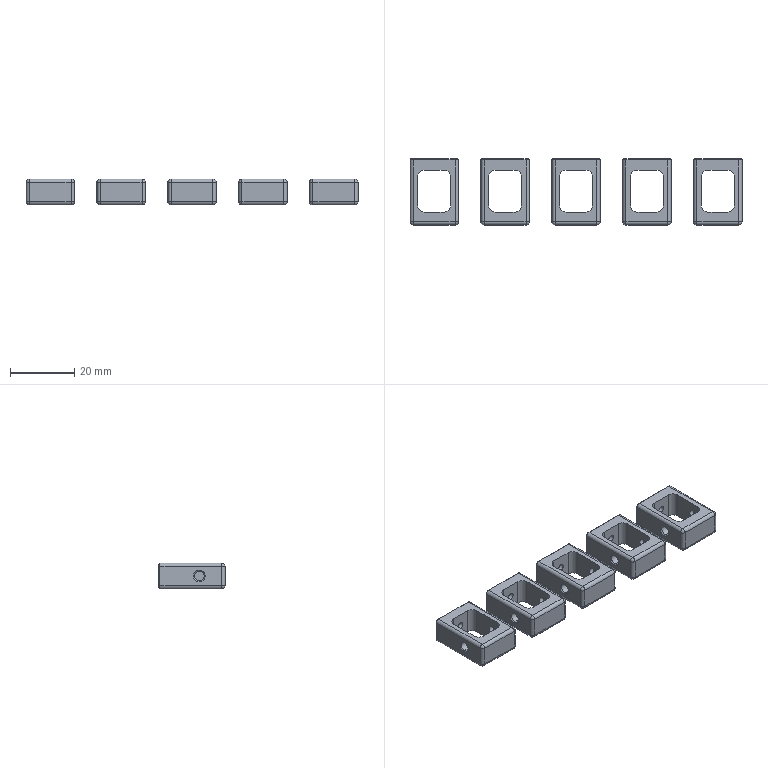NC program | NX | posted with a generic post | part box 103 x 20.5 x 8 mm
Lines 19 to 1022 of 9732:
(ZLEVEL_PROFILE , TOOL : D6)
N36 T12 M6
N38 G54
N40 G17 G0 G90 X20.275 Y-3.15 S9500 M3
N42 G43 Z30. H12
N44 Z1.5
N46 G94 G1 X24. Z1.305 F1000.
N48 Y3.65 Z0.948
N50 X20. Z0.739
N52 Y-3.15 Z0.382
N54 X24. Z0.173
N56 Y3.65 Z-0.184
N58 X20. Z-0.393
N60 Y0.25 Z-0.571
N62 Y-3.15 F3000.
N64 X24.
N66 Y3.65
N68 X20.
N70 Y0.25
N72 Y-3.15 Z-0.661
N74 X24. Z-0.767
N76 Y3.65 Z-0.947
N78 X20. Z-1.053
N80 Y0.25 Z-1.143
N82 Y-3.15 Z-1.233
N84 X24. Z-1.339
N86 Y3.65 Z-1.519
N88 X20. Z-1.624
N90 Y0.25 Z-1.714
N92 Y-3.15 Z-1.804
N94 X24. Z-1.91
N96 Y3.65 Z-2.09
N98 X20. Z-2.196
N100 Y0.25 Z-2.286
N102 Y-3.15 Z-2.376
N104 X24. Z-2.481
N106 Y3.65 Z-2.661
N108 X20. Z-2.767
N110 Y0.25 Z-2.857
N112 Y-3.15 Z-2.947
N114 X24. Z-3.053
N116 Y3.65 Z-3.233
N118 X20. Z-3.339
N120 Y0.25 Z-3.429
N122 Y-3.15 Z-3.519
N124 X24. Z-3.624
N126 Y3.65 Z-3.804
N128 X20. Z-3.91
N130 Y0.25 Z-4.
N132 Y-3.15 Z-4.09
N134 X24. Z-4.196
N136 Y3.65 Z-4.376
N138 X20. Z-4.481
N140 Y0.25 Z-4.571
N142 Y-3.15 Z-4.661
N144 X24. Z-4.767
N146 Y3.65 Z-4.947
N148 X20. Z-5.053
N150 Y0.25 Z-5.143
N152 Y-3.15 Z-5.233
N154 X24. Z-5.339
N156 Y3.65 Z-5.519
N158 X20. Z-5.624
N160 Y0.25 Z-5.714
N162 Y-3.15 Z-5.804
N164 X24. Z-5.91
N166 Y3.65 Z-6.09
N168 X20. Z-6.196
N170 Y0.25 Z-6.286
N172 Y-3.15 Z-6.376
N174 X24. Z-6.481
N176 Y3.65 Z-6.661
N178 X20. Z-6.767
N180 Y0.25 Z-6.857
N182 Y-3.15 Z-6.947
N184 X24. Z-7.053
N186 Y3.65 Z-7.233
N188 X20. Z-7.339
N190 Y0.25 Z-7.429
N192 Y-3.15 Z-7.519
N194 X24. Z-7.624
N196 Y3.65 Z-7.804
N198 X20. Z-7.91
N200 Y0.25 Z-8.
N202 Y-3.15
N204 X24.
N206 Y3.65
N208 X20.
N210 Y0.25
N212 Z-6.5
N214 G0 Z53.
N216 X1.725 Y3.65
N218 Z1.5
N220 G1 X-2. Z1.305 F1000.
N222 Y-3.15 Z0.948
N224 X2. Z0.739
N226 Y3.65 Z0.382
N228 X-2. Z0.173
N230 Y-3.15 Z-0.184
N232 X2. Z-0.393
N234 Y0.25 Z-0.571
N236 Y3.65 F3000.
N238 X-2.
N240 Y-3.15
N242 X2.
N244 Y0.25
N246 Y3.65 Z-0.661
N248 X-2. Z-0.767
N250 Y-3.15 Z-0.947
N252 X2. Z-1.053
N254 Y0.25 Z-1.143
N256 Y3.65 Z-1.233
N258 X-2. Z-1.339
N260 Y-3.15 Z-1.519
N262 X2. Z-1.624
N264 Y0.25 Z-1.714
N266 Y3.65 Z-1.804
N268 X-2. Z-1.91
N270 Y-3.15 Z-2.09
N272 X2. Z-2.196
N274 Y0.25 Z-2.286
N276 Y3.65 Z-2.376
N278 X-2. Z-2.481
N280 Y-3.15 Z-2.661
N282 X2. Z-2.767
N284 Y0.25 Z-2.857
N286 Y3.65 Z-2.947
N288 X-2. Z-3.053
N290 Y-3.15 Z-3.233
N292 X2. Z-3.339
N294 Y0.25 Z-3.429
N296 Y3.65 Z-3.519
N298 X-2. Z-3.624
N300 Y-3.15 Z-3.804
N302 X2. Z-3.91
N304 Y0.25 Z-4.
N306 Y3.65 Z-4.09
N308 X-2. Z-4.196
N310 Y-3.15 Z-4.376
N312 X2. Z-4.481
N314 Y0.25 Z-4.571
N316 Y3.65 Z-4.661
N318 X-2. Z-4.767
N320 Y-3.15 Z-4.947
N322 X2. Z-5.053
N324 Y0.25 Z-5.143
N326 Y3.65 Z-5.233
N328 X-2. Z-5.339
N330 Y-3.15 Z-5.519
N332 X2. Z-5.624
N334 Y0.25 Z-5.714
N336 Y3.65 Z-5.804
N338 X-2. Z-5.91
N340 Y-3.15 Z-6.09
N342 X2. Z-6.196
N344 Y0.25 Z-6.286
N346 Y3.65 Z-6.376
N348 X-2. Z-6.481
N350 Y-3.15 Z-6.661
N352 X2. Z-6.767
N354 Y0.25 Z-6.857
N356 Y3.65 Z-6.947
N358 X-2. Z-7.053
N360 Y-3.15 Z-7.233
N362 X2. Z-7.339
N364 Y0.25 Z-7.429
N366 Y3.65 Z-7.519
N368 X-2. Z-7.624
N370 Y-3.15 Z-7.804
N372 X2. Z-7.91
N374 Y0.25 Z-8.
N376 Y3.65
N378 X-2.
N380 Y-3.15
N382 X2.
N384 Y0.25
N386 Z-6.5
N388 G0 Z53.
N390 X-20.275 Y3.65
N392 Z1.5
N394 G1 X-24. Z1.305 F1000.
N396 Y-3.15 Z0.948
N398 X-20. Z0.739
N400 Y3.65 Z0.382
N402 X-24. Z0.173
N404 Y-3.15 Z-0.184
N406 X-20. Z-0.393
N408 Y0.25 Z-0.571
N410 Y3.65 F3000.
N412 X-24.
N414 Y-3.15
N416 X-20.
N418 Y0.25
N420 Y3.65 Z-0.661
N422 X-24. Z-0.767
N424 Y-3.15 Z-0.947
N426 X-20. Z-1.053
N428 Y0.25 Z-1.143
N430 Y3.65 Z-1.233
N432 X-24. Z-1.339
N434 Y-3.15 Z-1.519
N436 X-20. Z-1.624
N438 Y0.25 Z-1.714
N440 Y3.65 Z-1.804
N442 X-24. Z-1.91
N444 Y-3.15 Z-2.09
N446 X-20. Z-2.196
N448 Y0.25 Z-2.286
N450 Y3.65 Z-2.376
N452 X-24. Z-2.481
N454 Y-3.15 Z-2.661
N456 X-20. Z-2.767
N458 Y0.25 Z-2.857
N460 Y3.65 Z-2.947
N462 X-24. Z-3.053
N464 Y-3.15 Z-3.233
N466 X-20. Z-3.339
N468 Y0.25 Z-3.429
N470 Y3.65 Z-3.519
N472 X-24. Z-3.624
N474 Y-3.15 Z-3.804
N476 X-20. Z-3.91
N478 Y0.25 Z-4.
N480 Y3.65 Z-4.09
N482 X-24. Z-4.196
N484 Y-3.15 Z-4.376
N486 X-20. Z-4.481
N488 Y0.25 Z-4.571
N490 Y3.65 Z-4.661
N492 X-24. Z-4.767
N494 Y-3.15 Z-4.947
N496 X-20. Z-5.053
N498 Y0.25 Z-5.143
N500 Y3.65 Z-5.233
N502 X-24. Z-5.339
N504 Y-3.15 Z-5.519
N506 X-20. Z-5.624
N508 Y0.25 Z-5.714
N510 Y3.65 Z-5.804
N512 X-24. Z-5.91
N514 Y-3.15 Z-6.09
N516 X-20. Z-6.196
N518 Y0.25 Z-6.286
N520 Y3.65 Z-6.376
N522 X-24. Z-6.481
N524 Y-3.15 Z-6.661
N526 X-20. Z-6.767
N528 Y0.25 Z-6.857
N530 Y3.65 Z-6.947
N532 X-24. Z-7.053
N534 Y-3.15 Z-7.233
N536 X-20. Z-7.339
N538 Y0.25 Z-7.429
N540 Y3.65 Z-7.519
N542 X-24. Z-7.624
N544 Y-3.15 Z-7.804
N546 X-20. Z-7.91
N548 Y0.25 Z-8.
N550 Y3.65
N552 X-24.
N554 Y-3.15
N556 X-20.
N558 Y0.25
N560 Z-6.5
N562 G0 Z53.
N564 X-45.725 Y-3.15
N566 Z1.5
N568 G1 X-42. Z1.305 F1000.
N570 Y3.65 Z0.948
N572 X-46. Z0.739
N574 Y-3.15 Z0.382
N576 X-42. Z0.173
N578 Y3.65 Z-0.184
N580 X-46. Z-0.393
N582 Y0.25 Z-0.571
N584 Y-3.15 F3000.
N586 X-42.
N588 Y3.65
N590 X-46.
N592 Y0.25
N594 Y-3.15 Z-0.661
N596 X-42. Z-0.767
N598 Y3.65 Z-0.947
N600 X-46. Z-1.053
N602 Y0.25 Z-1.143
N604 Y-3.15 Z-1.233
N606 X-42. Z-1.339
N608 Y3.65 Z-1.519
N610 X-46. Z-1.624
N612 Y0.25 Z-1.714
N614 Y-3.15 Z-1.804
N616 X-42. Z-1.91
N618 Y3.65 Z-2.09
N620 X-46. Z-2.196
N622 Y0.25 Z-2.286
N624 Y-3.15 Z-2.376
N626 X-42. Z-2.481
N628 Y3.65 Z-2.661
N630 X-46. Z-2.767
N632 Y0.25 Z-2.857
N634 Y-3.15 Z-2.947
N636 X-42. Z-3.053
N638 Y3.65 Z-3.233
N640 X-46. Z-3.339
N642 Y0.25 Z-3.429
N644 Y-3.15 Z-3.519
N646 X-42. Z-3.624
N648 Y3.65 Z-3.804
N650 X-46. Z-3.91
N652 Y0.25 Z-4.
N654 Y-3.15 Z-4.09
N656 X-42. Z-4.196
N658 Y3.65 Z-4.376
N660 X-46. Z-4.481
N662 Y0.25 Z-4.571
N664 Y-3.15 Z-4.661
N666 X-42. Z-4.767
N668 Y3.65 Z-4.947
N670 X-46. Z-5.053
N672 Y0.25 Z-5.143
N674 Y-3.15 Z-5.233
N676 X-42. Z-5.339
N678 Y3.65 Z-5.519
N680 X-46. Z-5.624
N682 Y0.25 Z-5.714
N684 Y-3.15 Z-5.804
N686 X-42. Z-5.91
N688 Y3.65 Z-6.09
N690 X-46. Z-6.196
N692 Y0.25 Z-6.286
N694 Y-3.15 Z-6.376
N696 X-42. Z-6.481
N698 Y3.65 Z-6.661
N700 X-46. Z-6.767
N702 Y0.25 Z-6.857
N704 Y-3.15 Z-6.947
N706 X-42. Z-7.053
N708 Y3.65 Z-7.233
N710 X-46. Z-7.339
N712 Y0.25 Z-7.429
N714 Y-3.15 Z-7.519
N716 X-42. Z-7.624
N718 Y3.65 Z-7.804
N720 X-46. Z-7.91
N722 Y0.25 Z-8.
N724 Y-3.15
N726 X-42.
N728 Y3.65
N730 X-46.
N732 Y0.25
N734 Z-6.5
N736 G0 Z53.
N738 X45.725 Y3.65
N740 Z1.5
N742 G1 X42. Z1.305 F1000.
N744 Y-3.15 Z0.948
N746 X46. Z0.739
N748 Y3.65 Z0.382
N750 X42. Z0.173
N752 Y-3.15 Z-0.184
N754 X46. Z-0.393
N756 Y0.25 Z-0.571
N758 Y3.65 F3000.
N760 X42.
N762 Y-3.15
N764 X46.
N766 Y0.25
N768 Y3.65 Z-0.661
N770 X42. Z-0.767
N772 Y-3.15 Z-0.947
N774 X46. Z-1.053
N776 Y0.25 Z-1.143
N778 Y3.65 Z-1.233
N780 X42. Z-1.339
N782 Y-3.15 Z-1.519
N784 X46. Z-1.624
N786 Y0.25 Z-1.714
N788 Y3.65 Z-1.804
N790 X42. Z-1.91
N792 Y-3.15 Z-2.09
N794 X46. Z-2.196
N796 Y0.25 Z-2.286
N798 Y3.65 Z-2.376
N800 X42. Z-2.481
N802 Y-3.15 Z-2.661
N804 X46. Z-2.767
N806 Y0.25 Z-2.857
N808 Y3.65 Z-2.947
N810 X42. Z-3.053
N812 Y-3.15 Z-3.233
N814 X46. Z-3.339
N816 Y0.25 Z-3.429
N818 Y3.65 Z-3.519
N820 X42. Z-3.624
N822 Y-3.15 Z-3.804
N824 X46. Z-3.91
N826 Y0.25 Z-4.
N828 Y3.65 Z-4.09
N830 X42. Z-4.196
N832 Y-3.15 Z-4.376
N834 X46. Z-4.481
N836 Y0.25 Z-4.571
N838 Y3.65 Z-4.661
N840 X42. Z-4.767
N842 Y-3.15 Z-4.947
N844 X46. Z-5.053
N846 Y0.25 Z-5.143
N848 Y3.65 Z-5.233
N850 X42. Z-5.339
N852 Y-3.15 Z-5.519
N854 X46. Z-5.624
N856 Y0.25 Z-5.714
N858 Y3.65 Z-5.804
N860 X42. Z-5.91
N862 Y-3.15 Z-6.09
N864 X46. Z-6.196
N866 Y0.25 Z-6.286
N868 Y3.65 Z-6.376
N870 X42. Z-6.481
N872 Y-3.15 Z-6.661
N874 X46. Z-6.767
N876 Y0.25 Z-6.857
N878 Y3.65 Z-6.947
N880 X42. Z-7.053
N882 Y-3.15 Z-7.233
N884 X46. Z-7.339
N886 Y0.25 Z-7.429
N888 Y3.65 Z-7.519
N890 X42. Z-7.624
N892 Y-3.15 Z-7.804
N894 X46. Z-7.91
N896 Y0.25 Z-8.
N898 Y3.65
N900 X42.
N902 Y-3.15
N904 X46.
N906 Y0.25
N908 Z-6.5
N910 G0 Z53.
N912 X33.4 Y5.088
N914 Z1.5
N916 G1 Y9.95 Z1.245 F1000.
N918 X33.397 Y10.384 Z1.222
N920 X33.686 Y11.35 Z1.17
N922 X34.265 Y12.175 Z1.117
N924 X34.608 Y12.442 Z1.094
N926 X34.914 Y12.748 Z1.071
N928 X35.602 Y13.142 Z1.03
N930 X36.368 Y13.35 Z0.988
N932 X51.632 Z0.188
N934 X52.398 Y13.142 Z0.147
N936 X53.086 Y12.748 Z0.105
N938 X53.998 Y11.836 Z0.037
N940 X54.392 Y11.148 Z-0.004
N942 X54.6 Y10.382 Z-0.046
N944 Y0.35 Z-0.571
N946 Y-9.25 F3000.
N948 G2 X50.5 Y-13.35 R4.1
N950 G1 X37.5
N952 G2 X33.4 Y-9.25 R4.1
N954 G1 Y9.95
N956 G2 X34.608 Y12.442 R3.129
N958 X36.8 Y13.35 R3.1
N960 G1 X51.2
N962 G2 X53.392 Y12.442 R3.1
N964 G1 X53.692 Y12.142
N966 G2 X54.6 Y9.95 R3.1
N968 G1 Y0.35
N970 Y-9.25 Z-0.633
N972 X54.574 Y-9.709 Z-0.636
N974 X54.497 Y-10.162 Z-0.639
N976 X54.37 Y-10.604 Z-0.642
N978 X54.194 Y-11.029 Z-0.645
N980 X53.972 Y-11.431 Z-0.648
N982 X53.706 Y-11.806 Z-0.651
N984 X53.399 Y-12.149 Z-0.653
N986 X53.056 Y-12.456 Z-0.656
N988 X52.681 Y-12.722 Z-0.659
N990 X52.279 Y-12.944 Z-0.662
N992 X51.854 Y-13.12 Z-0.665
N994 X51.412 Y-13.247 Z-0.668
N996 X50.959 Y-13.324 Z-0.671
N998 X50.5 Y-13.35 Z-0.674
N1000 X37.5 Z-0.757
N1002 X37.041 Y-13.324 Z-0.76
N1004 X36.588 Y-13.247 Z-0.763
N1006 X36.146 Y-13.12 Z-0.766
N1008 X35.721 Y-12.944 Z-0.769
N1010 X35.319 Y-12.722 Z-0.772
N1012 X34.944 Y-12.456 Z-0.775
N1014 X34.601 Y-12.149 Z-0.778
N1016 X34.294 Y-11.806 Z-0.781
N1018 X34.028 Y-11.431 Z-0.784
N1020 X33.806 Y-11.029 Z-0.787
N1022 X33.63 Y-10.604 Z-0.79
N1024 X33.503 Y-10.162 Z-0.793
N1026 X33.426 Y-9.709 Z-0.796
N1028 X33.4 Y-9.25 Z-0.798
N1030 Y9.95 Z-0.921
N1032 X33.421 Y10.307 Z-0.924
N1034 X33.482 Y10.66 Z-0.926
N1036 X33.584 Y11.003 Z-0.928
N1038 X33.725 Y11.331 Z-0.931
N1040 X33.902 Y11.641 Z-0.933
N1042 X34.113 Y11.928 Z-0.935
N1044 X34.356 Y12.19 Z-0.937
N1046 X34.608 Y12.442 Z-0.94
N1048 X34.913 Y12.71 Z-0.942
N1050 X35.25 Y12.935 Z-0.945
N1052 X35.614 Y13.114 Z-0.948
N1054 X35.998 Y13.244 Z-0.95
N1056 X36.395 Y13.323 Z-0.953
N1058 X36.8 Y13.35 Z-0.955
N1060 X51.2 Z-1.048
N1062 X51.605 Y13.323 Z-1.05
N1064 X52.002 Y13.244 Z-1.053
N1066 X52.386 Y13.114 Z-1.055
N1068 X52.75 Y12.935 Z-1.058
N1070 X53.087 Y12.709 Z-1.061
N1072 X53.392 Y12.442 Z-1.063
N1074 X53.692 Y12.142 Z-1.066
N1076 X53.959 Y11.837 Z-1.068
N1078 X54.185 Y11.5 Z-1.071
N1080 X54.364 Y11.136 Z-1.074
N1082 X54.494 Y10.752 Z-1.076
N1084 X54.573 Y10.355 Z-1.079
N1086 X54.6 Y9.95 Z-1.081
N1088 Y0.35 Z-1.143
N1090 Y-9.25 Z-1.204
N1092 X54.574 Y-9.709 Z-1.207
N1094 X54.497 Y-10.162 Z-1.21
N1096 X54.37 Y-10.604 Z-1.213
N1098 X54.194 Y-11.029 Z-1.216
N1100 X53.972 Y-11.431 Z-1.219
N1102 X53.706 Y-11.806 Z-1.222
N1104 X53.399 Y-12.149 Z-1.225
N1106 X53.056 Y-12.456 Z-1.228
N1108 X52.681 Y-12.722 Z-1.231
N1110 X52.279 Y-12.944 Z-1.234
N1112 X51.854 Y-13.12 Z-1.237
N1114 X51.412 Y-13.247 Z-1.24
N1116 X50.959 Y-13.324 Z-1.243
N1118 X50.5 Y-13.35 Z-1.246
N1120 X37.5 Z-1.329
N1122 X37.041 Y-13.324 Z-1.332
N1124 X36.588 Y-13.247 Z-1.335
N1126 X36.146 Y-13.12 Z-1.338
N1128 X35.721 Y-12.944 Z-1.341
N1130 X35.319 Y-12.722 Z-1.343
N1132 X34.944 Y-12.456 Z-1.346
N1134 X34.601 Y-12.149 Z-1.349
N1136 X34.294 Y-11.806 Z-1.352
N1138 X34.028 Y-11.431 Z-1.355
N1140 X33.806 Y-11.029 Z-1.358
N1142 X33.63 Y-10.604 Z-1.361
N1144 X33.503 Y-10.162 Z-1.364
N1146 X33.426 Y-9.709 Z-1.367
N1148 X33.4 Y-9.25 Z-1.37
N1150 Y9.95 Z-1.493
N1152 X33.421 Y10.307 Z-1.495
N1154 X33.482 Y10.66 Z-1.497
N1156 X33.584 Y11.003 Z-1.5
N1158 X33.725 Y11.331 Z-1.502
N1160 X33.902 Y11.641 Z-1.504
N1162 X34.113 Y11.928 Z-1.507
N1164 X34.356 Y12.19 Z-1.509
N1166 X34.608 Y12.442 Z-1.511
N1168 X34.913 Y12.71 Z-1.514
N1170 X35.25 Y12.935 Z-1.516
N1172 X35.614 Y13.114 Z-1.519
N1174 X35.998 Y13.244 Z-1.522
N1176 X36.395 Y13.323 Z-1.524
N1178 X36.8 Y13.35 Z-1.527
N1180 X51.2 Z-1.619
N1182 X51.605 Y13.323 Z-1.622
N1184 X52.002 Y13.244 Z-1.624
N1186 X52.386 Y13.114 Z-1.627
N1188 X52.75 Y12.935 Z-1.629
N1190 X53.087 Y12.709 Z-1.632
N1192 X53.392 Y12.442 Z-1.635
N1194 X53.692 Y12.142 Z-1.637
N1196 X53.959 Y11.837 Z-1.64
N1198 X54.185 Y11.5 Z-1.642
N1200 X54.364 Y11.136 Z-1.645
N1202 X54.494 Y10.752 Z-1.648
N1204 X54.573 Y10.355 Z-1.65
N1206 X54.6 Y9.95 Z-1.653
N1208 Y0.35 Z-1.714
N1210 Y-9.25 Z-1.776
N1212 X54.574 Y-9.709 Z-1.779
N1214 X54.497 Y-10.162 Z-1.782
N1216 X54.37 Y-10.604 Z-1.785
N1218 X54.194 Y-11.029 Z-1.788
N1220 X53.972 Y-11.431 Z-1.79
N1222 X53.706 Y-11.806 Z-1.793
N1224 X53.399 Y-12.149 Z-1.796
N1226 X53.056 Y-12.456 Z-1.799
N1228 X52.681 Y-12.722 Z-1.802
N1230 X52.279 Y-12.944 Z-1.805
N1232 X51.854 Y-13.12 Z-1.808
N1234 X51.412 Y-13.247 Z-1.811
N1236 X50.959 Y-13.324 Z-1.814
N1238 X50.5 Y-13.35 Z-1.817
N1240 X37.5 Z-1.9
N1242 X37.041 Y-13.324 Z-1.903
N1244 X36.588 Y-13.247 Z-1.906
N1246 X36.146 Y-13.12 Z-1.909
N1248 X35.721 Y-12.944 Z-1.912
N1250 X35.319 Y-12.722 Z-1.915
N1252 X34.944 Y-12.456 Z-1.918
N1254 X34.601 Y-12.149 Z-1.921
N1256 X34.294 Y-11.806 Z-1.924
N1258 X34.028 Y-11.431 Z-1.927
N1260 X33.806 Y-11.029 Z-1.93
N1262 X33.63 Y-10.604 Z-1.933
N1264 X33.503 Y-10.162 Z-1.935
N1266 X33.426 Y-9.709 Z-1.938
N1268 X33.4 Y-9.25 Z-1.941
N1270 Y9.95 Z-2.064
N1272 X33.421 Y10.307 Z-2.067
N1274 X33.482 Y10.66 Z-2.069
N1276 X33.584 Y11.003 Z-2.071
N1278 X33.725 Y11.331 Z-2.073
N1280 X33.902 Y11.641 Z-2.076
N1282 X34.113 Y11.928 Z-2.078
N1284 X34.356 Y12.19 Z-2.08
N1286 X34.608 Y12.442 Z-2.083
N1288 X34.913 Y12.71 Z-2.085
N1290 X35.25 Y12.935 Z-2.088
N1292 X35.614 Y13.114 Z-2.09
N1294 X35.998 Y13.244 Z-2.093
N1296 X36.395 Y13.323 Z-2.096
N1298 X36.8 Y13.35 Z-2.098
N1300 X51.2 Z-2.19
N1302 X51.605 Y13.323 Z-2.193
N1304 X52.002 Y13.244 Z-2.196
N1306 X52.386 Y13.114 Z-2.198
N1308 X52.75 Y12.935 Z-2.201
N1310 X53.087 Y12.709 Z-2.203
N1312 X53.392 Y12.442 Z-2.206
N1314 X53.692 Y12.142 Z-2.209
N1316 X53.959 Y11.837 Z-2.211
N1318 X54.185 Y11.5 Z-2.214
N1320 X54.364 Y11.136 Z-2.216
N1322 X54.494 Y10.752 Z-2.219
N1324 X54.573 Y10.355 Z-2.222
N1326 X54.6 Y9.95 Z-2.224
N1328 Y0.35 Z-2.286
N1330 Y-9.25 Z-2.347
N1332 X54.574 Y-9.709 Z-2.35
N1334 X54.497 Y-10.162 Z-2.353
N1336 X54.37 Y-10.604 Z-2.356
N1338 X54.194 Y-11.029 Z-2.359
N1340 X53.972 Y-11.431 Z-2.362
N1342 X53.706 Y-11.806 Z-2.365
N1344 X53.399 Y-12.149 Z-2.368
N1346 X53.056 Y-12.456 Z-2.371
N1348 X52.681 Y-12.722 Z-2.374
N1350 X52.279 Y-12.944 Z-2.377
N1352 X51.854 Y-13.12 Z-2.38
N1354 X51.412 Y-13.247 Z-2.382
N1356 X50.959 Y-13.324 Z-2.385
N1358 X50.5 Y-13.35 Z-2.388
N1360 X37.5 Z-2.472
N1362 X37.041 Y-13.324 Z-2.475
N1364 X36.588 Y-13.247 Z-2.477
N1366 X36.146 Y-13.12 Z-2.48
N1368 X35.721 Y-12.944 Z-2.483
N1370 X35.319 Y-12.722 Z-2.486
N1372 X34.944 Y-12.456 Z-2.489
N1374 X34.601 Y-12.149 Z-2.492
N1376 X34.294 Y-11.806 Z-2.495
N1378 X34.028 Y-11.431 Z-2.498
N1380 X33.806 Y-11.029 Z-2.501
N1382 X33.63 Y-10.604 Z-2.504
N1384 X33.503 Y-10.162 Z-2.507
N1386 X33.426 Y-9.709 Z-2.51
N1388 X33.4 Y-9.25 Z-2.513
N1390 Y9.95 Z-2.636
N1392 X33.421 Y10.307 Z-2.638
N1394 X33.482 Y10.66 Z-2.64
N1396 X33.584 Y11.003 Z-2.643
N1398 X33.725 Y11.331 Z-2.645
N1400 X33.902 Y11.641 Z-2.647
N1402 X34.113 Y11.928 Z-2.649
N1404 X34.356 Y12.19 Z-2.652
N1406 X34.608 Y12.442 Z-2.654
N1408 X34.913 Y12.71 Z-2.657
N1410 X35.25 Y12.935 Z-2.659
N1412 X35.614 Y13.114 Z-2.662
N1414 X35.998 Y13.244 Z-2.664
N1416 X36.395 Y13.323 Z-2.667
N1418 X36.8 Y13.35 Z-2.67
N1420 X51.2 Z-2.762
N1422 X51.605 Y13.323 Z-2.764
N1424 X52.002 Y13.244 Z-2.767
N1426 X52.386 Y13.114 Z-2.77
N1428 X52.75 Y12.935 Z-2.772
N1430 X53.087 Y12.709 Z-2.775
N1432 X53.392 Y12.442 Z-2.777
N1434 X53.692 Y12.142 Z-2.78
N1436 X53.959 Y11.837 Z-2.783
N1438 X54.185 Y11.5 Z-2.785
N1440 X54.364 Y11.136 Z-2.788
N1442 X54.494 Y10.752 Z-2.79
N1444 X54.573 Y10.355 Z-2.793
N1446 X54.6 Y9.95 Z-2.796
N1448 Y0.35 Z-2.857
N1450 Y-9.25 Z-2.919
N1452 X54.574 Y-9.709 Z-2.922
N1454 X54.497 Y-10.162 Z-2.925
N1456 X54.37 Y-10.604 Z-2.927
N1458 X54.194 Y-11.029 Z-2.93
N1460 X53.972 Y-11.431 Z-2.933
N1462 X53.706 Y-11.806 Z-2.936
N1464 X53.399 Y-12.149 Z-2.939
N1466 X53.056 Y-12.456 Z-2.942
N1468 X52.681 Y-12.722 Z-2.945
N1470 X52.279 Y-12.944 Z-2.948
N1472 X51.854 Y-13.12 Z-2.951
N1474 X51.412 Y-13.247 Z-2.954
N1476 X50.959 Y-13.324 Z-2.957
N1478 X50.5 Y-13.35 Z-2.96
N1480 X37.5 Z-3.043
N1482 X37.041 Y-13.324 Z-3.046
N1484 X36.588 Y-13.247 Z-3.049
N1486 X36.146 Y-13.12 Z-3.052
N1488 X35.721 Y-12.944 Z-3.055
N1490 X35.319 Y-12.722 Z-3.058
N1492 X34.944 Y-12.456 Z-3.061
N1494 X34.601 Y-12.149 Z-3.064
N1496 X34.294 Y-11.806 Z-3.067
N1498 X34.028 Y-11.431 Z-3.07
N1500 X33.806 Y-11.029 Z-3.072
N1502 X33.63 Y-10.604 Z-3.075
N1504 X33.503 Y-10.162 Z-3.078
N1506 X33.426 Y-9.709 Z-3.081
N1508 X33.4 Y-9.25 Z-3.084
N1510 Y9.95 Z-3.207
N1512 X33.421 Y10.307 Z-3.209
N1514 X33.482 Y10.66 Z-3.212
N1516 X33.584 Y11.003 Z-3.214
N1518 X33.725 Y11.331 Z-3.216
N1520 X33.902 Y11.641 Z-3.219
N1522 X34.113 Y11.928 Z-3.221
N1524 X34.356 Y12.19 Z-3.223
N1526 X34.608 Y12.442 Z-3.226
N1528 X34.913 Y12.71 Z-3.228
N1530 X35.25 Y12.935 Z-3.231
N1532 X35.614 Y13.114 Z-3.233
N1534 X35.998 Y13.244 Z-3.236
N1536 X36.395 Y13.323 Z-3.238
N1538 X36.8 Y13.35 Z-3.241
N1540 X51.2 Z-3.333
N1542 X51.605 Y13.323 Z-3.336
N1544 X52.002 Y13.244 Z-3.338
N1546 X52.386 Y13.114 Z-3.341
N1548 X52.75 Y12.935 Z-3.344
N1550 X53.087 Y12.709 Z-3.346
N1552 X53.392 Y12.442 Z-3.349
N1554 X53.692 Y12.142 Z-3.352
N1556 X53.959 Y11.837 Z-3.354
N1558 X54.185 Y11.5 Z-3.357
N1560 X54.364 Y11.136 Z-3.359
N1562 X54.494 Y10.752 Z-3.362
N1564 X54.573 Y10.355 Z-3.364
N1566 X54.6 Y9.95 Z-3.367
N1568 Y0.35 Z-3.429
N1570 Y-9.25 Z-3.49
N1572 X54.574 Y-9.709 Z-3.493
N1574 X54.497 Y-10.162 Z-3.496
N1576 X54.37 Y-10.604 Z-3.499
N1578 X54.194 Y-11.029 Z-3.502
N1580 X53.972 Y-11.431 Z-3.505
N1582 X53.706 Y-11.806 Z-3.508
N1584 X53.399 Y-12.149 Z-3.511
N1586 X53.056 Y-12.456 Z-3.514
N1588 X52.681 Y-12.722 Z-3.517
N1590 X52.279 Y-12.944 Z-3.519
N1592 X51.854 Y-13.12 Z-3.522
N1594 X51.412 Y-13.247 Z-3.525
N1596 X50.959 Y-13.324 Z-3.528
N1598 X50.5 Y-13.35 Z-3.531
N1600 X37.5 Z-3.614
N1602 X37.041 Y-13.324 Z-3.617
N1604 X36.588 Y-13.247 Z-3.62
N1606 X36.146 Y-13.12 Z-3.623
N1608 X35.721 Y-12.944 Z-3.626
N1610 X35.319 Y-12.722 Z-3.629
N1612 X34.944 Y-12.456 Z-3.632
N1614 X34.601 Y-12.149 Z-3.635
N1616 X34.294 Y-11.806 Z-3.638
N1618 X34.028 Y-11.431 Z-3.641
N1620 X33.806 Y-11.029 Z-3.644
N1622 X33.63 Y-10.604 Z-3.647
N1624 X33.503 Y-10.162 Z-3.65
N1626 X33.426 Y-9.709 Z-3.653
N1628 X33.4 Y-9.25 Z-3.656
N1630 Y9.95 Z-3.779
N1632 X33.421 Y10.307 Z-3.781
N1634 X33.482 Y10.66 Z-3.783
N1636 X33.584 Y11.003 Z-3.785
N1638 X33.725 Y11.331 Z-3.788
N1640 X33.902 Y11.641 Z-3.79
N1642 X34.113 Y11.928 Z-3.792
N1644 X34.356 Y12.19 Z-3.795
N1646 X34.608 Y12.442 Z-3.797
N1648 X34.913 Y12.71 Z-3.8
N1650 X35.25 Y12.935 Z-3.802
N1652 X35.614 Y13.114 Z-3.805
N1654 X35.998 Y13.244 Z-3.807
N1656 X36.395 Y13.323 Z-3.81
N1658 X36.8 Y13.35 Z-3.812
N1660 X51.2 Z-3.905
N1662 X51.605 Y13.323 Z-3.907
N1664 X52.002 Y13.244 Z-3.91
N1666 X52.386 Y13.114 Z-3.912
N1668 X52.75 Y12.935 Z-3.915
N1670 X53.087 Y12.709 Z-3.918
N1672 X53.392 Y12.442 Z-3.92
N1674 X53.692 Y12.142 Z-3.923
N1676 X53.959 Y11.837 Z-3.926
N1678 X54.185 Y11.5 Z-3.928
N1680 X54.364 Y11.136 Z-3.931
N1682 X54.494 Y10.752 Z-3.933
N1684 X54.573 Y10.355 Z-3.936
N1686 X54.6 Y9.95 Z-3.939
N1688 Y0.35 Z-4.
N1690 Y-9.25 Z-4.061
N1692 X54.574 Y-9.709 Z-4.064
N1694 X54.497 Y-10.162 Z-4.067
N1696 X54.37 Y-10.604 Z-4.07
N1698 X54.194 Y-11.029 Z-4.073
N1700 X53.972 Y-11.431 Z-4.076
N1702 X53.706 Y-11.806 Z-4.079
N1704 X53.399 Y-12.149 Z-4.082
N1706 X53.056 Y-12.456 Z-4.085
N1708 X52.681 Y-12.722 Z-4.088
N1710 X52.279 Y-12.944 Z-4.091
N1712 X51.854 Y-13.12 Z-4.094
N1714 X51.412 Y-13.247 Z-4.097
N1716 X50.959 Y-13.324 Z-4.1
N1718 X50.5 Y-13.35 Z-4.103
N1720 X37.5 Z-4.186
N1722 X37.041 Y-13.324 Z-4.189
N1724 X36.588 Y-13.247 Z-4.192
N1726 X36.146 Y-13.12 Z-4.195
N1728 X35.721 Y-12.944 Z-4.198
N1730 X35.319 Y-12.722 Z-4.201
N1732 X34.944 Y-12.456 Z-4.204
N1734 X34.601 Y-12.149 Z-4.206
N1736 X34.294 Y-11.806 Z-4.209
N1738 X34.028 Y-11.431 Z-4.212
N1740 X33.806 Y-11.029 Z-4.215
N1742 X33.63 Y-10.604 Z-4.218
N1744 X33.503 Y-10.162 Z-4.221
N1746 X33.426 Y-9.709 Z-4.224
N1748 X33.4 Y-9.25 Z-4.227
N1750 Y9.95 Z-4.35
N1752 X33.421 Y10.307 Z-4.352
N1754 X33.482 Y10.66 Z-4.355
N1756 X33.584 Y11.003 Z-4.357
N1758 X33.725 Y11.331 Z-4.359
N1760 X33.902 Y11.641 Z-4.361
N1762 X34.113 Y11.928 Z-4.364
N1764 X34.356 Y12.19 Z-4.366
N1766 X34.608 Y12.442 Z-4.368
N1768 X34.913 Y12.71 Z-4.371
N1770 X35.25 Y12.935 Z-4.374
N1772 X35.614 Y13.114 Z-4.376
N1774 X35.998 Y13.244 Z-4.379
N1776 X36.395 Y13.323 Z-4.381
N1778 X36.8 Y13.35 Z-4.384
N1780 X51.2 Z-4.476
N1782 X51.605 Y13.323 Z-4.479
N1784 X52.002 Y13.244 Z-4.481
N1786 X52.386 Y13.114 Z-4.484
N1788 X52.75 Y12.935 Z-4.486
N1790 X53.087 Y12.709 Z-4.489
N1792 X53.392 Y12.442 Z-4.492
N1794 X53.692 Y12.142 Z-4.494
N1796 X53.959 Y11.837 Z-4.497
N1798 X54.185 Y11.5 Z-4.5
N1800 X54.364 Y11.136 Z-4.502
N1802 X54.494 Y10.752 Z-4.505
N1804 X54.573 Y10.355 Z-4.507
N1806 X54.6 Y9.95 Z-4.51
N1808 Y0.35 Z-4.571
N1810 Y-9.25 Z-4.633
N1812 X54.574 Y-9.709 Z-4.636
N1814 X54.497 Y-10.162 Z-4.639
N1816 X54.37 Y-10.604 Z-4.642
N1818 X54.194 Y-11.029 Z-4.645
N1820 X53.972 Y-11.431 Z-4.648
N1822 X53.706 Y-11.806 Z-4.651
N1824 X53.399 Y-12.149 Z-4.653
N1826 X53.056 Y-12.456 Z-4.656
N1828 X52.681 Y-12.722 Z-4.659
N1830 X52.279 Y-12.944 Z-4.662
N1832 X51.854 Y-13.12 Z-4.665
N1834 X51.412 Y-13.247 Z-4.668
N1836 X50.959 Y-13.324 Z-4.671
N1838 X50.5 Y-13.35 Z-4.674
N1840 X37.5 Z-4.757
N1842 X37.041 Y-13.324 Z-4.76
N1844 X36.588 Y-13.247 Z-4.763
N1846 X36.146 Y-13.12 Z-4.766
N1848 X35.721 Y-12.944 Z-4.769
N1850 X35.319 Y-12.722 Z-4.772
N1852 X34.944 Y-12.456 Z-4.775
N1854 X34.601 Y-12.149 Z-4.778
N1856 X34.294 Y-11.806 Z-4.781
N1858 X34.028 Y-11.431 Z-4.784
N1860 X33.806 Y-11.029 Z-4.787
N1862 X33.63 Y-10.604 Z-4.79
N1864 X33.503 Y-10.162 Z-4.793
N1866 X33.426 Y-9.709 Z-4.796
N1868 X33.4 Y-9.25 Z-4.798
N1870 Y9.95 Z-4.921
N1872 X33.421 Y10.307 Z-4.924
N1874 X33.482 Y10.66 Z-4.926
N1876 X33.584 Y11.003 Z-4.928
N1878 X33.725 Y11.331 Z-4.931
N1880 X33.902 Y11.641 Z-4.933
N1882 X34.113 Y11.928 Z-4.935
N1884 X34.356 Y12.19 Z-4.937
N1886 X34.608 Y12.442 Z-4.94
N1888 X34.913 Y12.71 Z-4.942
N1890 X35.25 Y12.935 Z-4.945
N1892 X35.614 Y13.114 Z-4.948
N1894 X35.998 Y13.244 Z-4.95
N1896 X36.395 Y13.323 Z-4.953
N1898 X36.8 Y13.35 Z-4.955
N1900 X51.2 Z-5.048
N1902 X51.605 Y13.323 Z-5.05
N1904 X52.002 Y13.244 Z-5.053
N1906 X52.386 Y13.114 Z-5.055
N1908 X52.75 Y12.935 Z-5.058
N1910 X53.087 Y12.709 Z-5.061
N1912 X53.392 Y12.442 Z-5.063
N1914 X53.692 Y12.142 Z-5.066
N1916 X53.959 Y11.837 Z-5.068
N1918 X54.185 Y11.5 Z-5.071
N1920 X54.364 Y11.136 Z-5.074
N1922 X54.494 Y10.752 Z-5.076
N1924 X54.573 Y10.355 Z-5.079
N1926 X54.6 Y9.95 Z-5.081
N1928 Y0.35 Z-5.143
N1930 Y-9.25 Z-5.204
N1932 X54.574 Y-9.709 Z-5.207
N1934 X54.497 Y-10.162 Z-5.21
N1936 X54.37 Y-10.604 Z-5.213
N1938 X54.194 Y-11.029 Z-5.216
N1940 X53.972 Y-11.431 Z-5.219
N1942 X53.706 Y-11.806 Z-5.222
N1944 X53.399 Y-12.149 Z-5.225
N1946 X53.056 Y-12.456 Z-5.228
N1948 X52.681 Y-12.722 Z-5.231
N1950 X52.279 Y-12.944 Z-5.234
N1952 X51.854 Y-13.12 Z-5.237
N1954 X51.412 Y-13.247 Z-5.24
N1956 X50.959 Y-13.324 Z-5.243
N1958 X50.5 Y-13.35 Z-5.246
N1960 X37.5 Z-5.329
N1962 X37.041 Y-13.324 Z-5.332
N1964 X36.588 Y-13.247 Z-5.335
N1966 X36.146 Y-13.12 Z-5.338
N1968 X35.721 Y-12.944 Z-5.341
N1970 X35.319 Y-12.722 Z-5.343
N1972 X34.944 Y-12.456 Z-5.346
N1974 X34.601 Y-12.149 Z-5.349
N1976 X34.294 Y-11.806 Z-5.352
N1978 X34.028 Y-11.431 Z-5.355
N1980 X33.806 Y-11.029 Z-5.358
N1982 X33.63 Y-10.604 Z-5.361
N1984 X33.503 Y-10.162 Z-5.364
N1986 X33.426 Y-9.709 Z-5.367
N1988 X33.4 Y-9.25 Z-5.37
N1990 Y9.95 Z-5.493
N1992 X33.421 Y10.307 Z-5.495
N1994 X33.482 Y10.66 Z-5.497
N1996 X33.584 Y11.003 Z-5.5
N1998 X33.725 Y11.331 Z-5.502
N2000 X33.902 Y11.641 Z-5.504
N2002 X34.113 Y11.928 Z-5.507
N2004 X34.356 Y12.19 Z-5.509
N2006 X34.608 Y12.442 Z-5.511
N2008 X34.913 Y12.71 Z-5.514
N2010 X35.25 Y12.935 Z-5.516
N2012 X35.614 Y13.114 Z-5.519
N2014 X35.998 Y13.244 Z-5.522
N2016 X36.395 Y13.323 Z-5.524
N2018 X36.8 Y13.35 Z-5.527
N2020 X51.2 Z-5.619
N2022 X51.605 Y13.323 Z-5.622
N2024 X52.002 Y13.244 Z-5.624
N2026 X52.386 Y13.114 Z-5.627
N2028 X52.75 Y12.935 Z-5.629
N2030 X53.087 Y12.709 Z-5.632
N2032 X53.392 Y12.442 Z-5.635
N2034 X53.692 Y12.142 Z-5.637
N2036 X53.959 Y11.837 Z-5.64